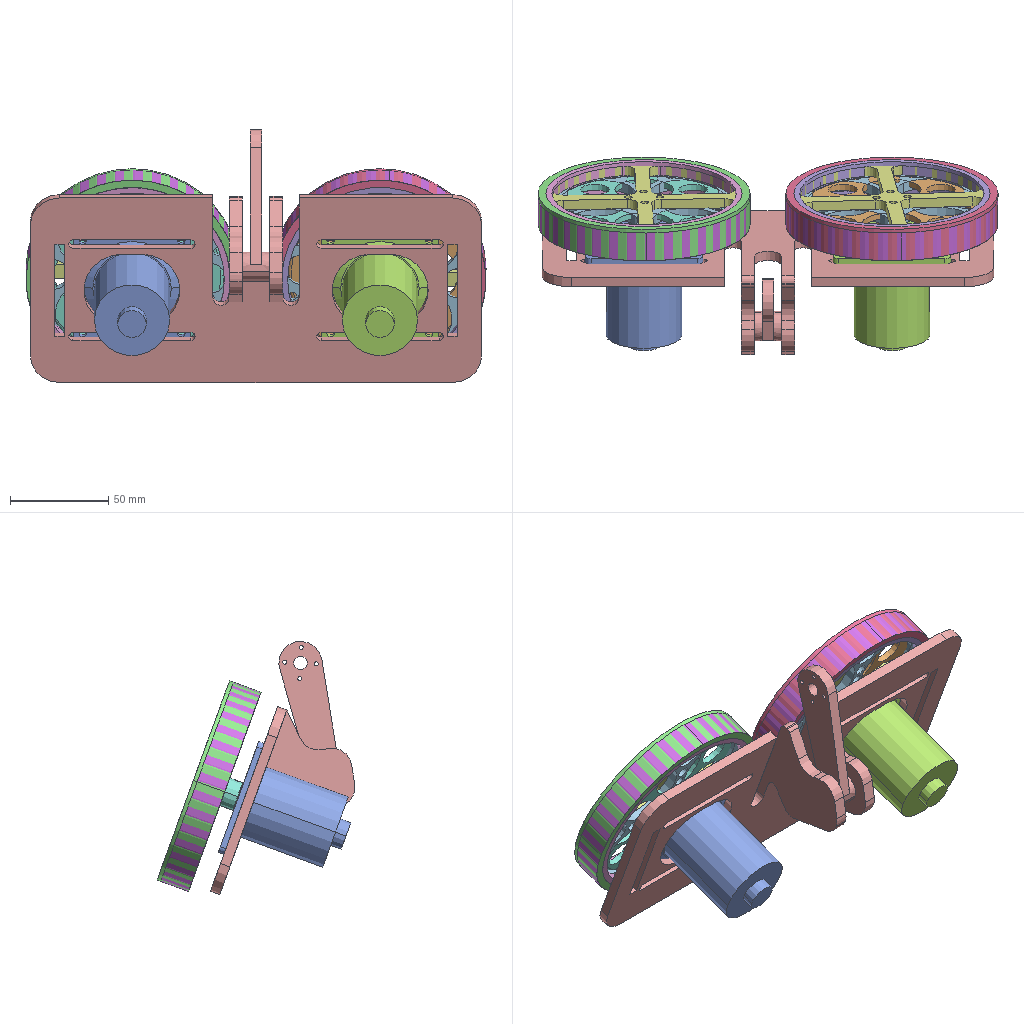Assembly | SolidWorks | 7 different items | 11 placed | box 234 x 101 x 129 mm
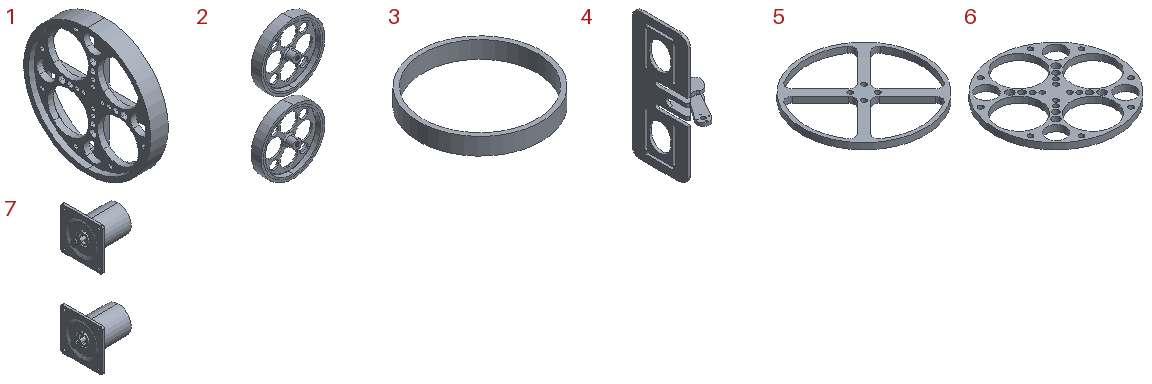Parts list (item | name | quantity | parent item | size | volume | features):
1 | (subassembly) | x2 | - | 15 x 108 x 108 mm | 45132 mm3 | -
2 | - | x1 | - | 108 x 24 x 234.2 mm | 99355 mm3 | features BaseBody 4, ICE 3
3 | - | x2 | in 1 | 108 x 108 x 15 mm | 19604 mm3 | features Extrusion 1
4 | - | x1 | - | 59.27 x 135.834 x 230 mm | 110956 mm3 | features ICE 12, Cut 3, Fillet 3, MirrorPattern 2, BaseBody 1
5 | - | x2 | in 1 | 100 x 100 x 5 mm | 11461 mm3 | features Cut 1, Extrusion 1, Fillet 1
6 | - | x2 | in 1 | 100 x 100 x 5 mm | 14067 mm3 | features CirPattern 3, ICE 3, Extrusion 1
7 | - | x1 | - | 70.7 x 60 x 186.2 mm | 133005 mm3 | features BaseBody 2
Mates (type | each side: item.copy, entity, surface, feature):
In the top assembly
Concentric | 7.1 face cylinder Imported1 | 3.1 face cylinder Boss-Extrude1
Coincident | 7.1 face plane Imported1 | 6.1 face plane Boss-Extrude1
Concentric | 7.1 face cylinder Imported2 | 3.2 face cylinder Boss-Extrude1
Coincident | 7.1 face plane Imported2 | 6.2 face plane Boss-Extrude1
In subassembly 1
Concentric | 3.3 face cylinder Boss-Extrude1 | 6.3 face cylinder Boss-Extrude1
InPlace | 6.3 face plane Boss-Extrude1 | 5.1 plane
Coincident | 5.1 face plane Boss-Extrude1 | 3.3 face plane Boss-Extrude1